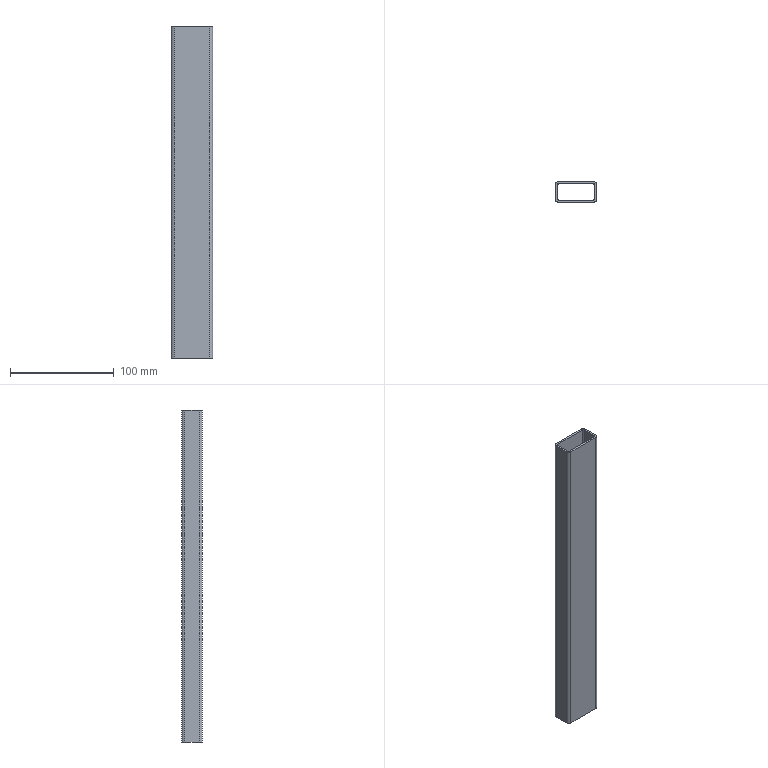Part | SolidWorks | features BaseBody 1 | 1 solid | 18 faces | box 40 x 20 x 320 mm | volume 69482 mm3 | plane 10 | cylinder 8 | commonest cylinder face diameters 2 x4 6 x4
STEP:
#1=CARTESIAN_POINT('',(18.,-7.,-160.));
#2=VERTEX_POINT('',#1);
#3=CARTESIAN_POINT('',(18.,7.,-160.));
#4=VERTEX_POINT('',#3);
#5=CARTESIAN_POINT('',(18.,7.,-160.));
#6=DIRECTION('',(0.,1.,0.));
#7=VECTOR('',#6,1000.);
#8=LINE('',#5,#7);
#9=EDGE_CURVE('',#2,#4,#8,.T.);
#10=ORIENTED_EDGE('',*,*,#9,.F.);
#11=CARTESIAN_POINT('',(18.,-7.,160.));
#12=VERTEX_POINT('',#11);
#13=CARTESIAN_POINT('',(18.,-7.,160.));
#14=DIRECTION('',(0.,0.,-1.));
#15=VECTOR('',#14,1000.);
#16=LINE('',#13,#15);
#17=EDGE_CURVE('',#12,#2,#16,.T.);
#18=ORIENTED_EDGE('',*,*,#17,.F.);
#19=CARTESIAN_POINT('',(18.,7.,160.));
#20=VERTEX_POINT('',#19);
#21=CARTESIAN_POINT('',(18.,7.,160.));
#22=DIRECTION('',(0.,1.,0.));
#23=VECTOR('',#22,1000.);
#24=LINE('',#21,#23);
#25=EDGE_CURVE('',#12,#20,#24,.T.);
#26=ORIENTED_EDGE('',*,*,#25,.T.);
#27=CARTESIAN_POINT('',(18.,7.,160.));
#28=DIRECTION('',(0.,0.,-1.));
#29=VECTOR('',#28,1000.);
#30=LINE('',#27,#29);
#31=EDGE_CURVE('',#20,#4,#30,.T.);
#32=ORIENTED_EDGE('',*,*,#31,.T.);
#33=EDGE_LOOP('',(#10,#18,#26,#32));
#34=FACE_OUTER_BOUND('',#33,.T.);
#35=CARTESIAN_POINT('',(18.,7.,160.));
#36=DIRECTION('',(-1.,0.,0.));
#37=DIRECTION('',(0.,0.,1.));
#38=AXIS2_PLACEMENT_3D('',#35,#36,#37);
#39=PLANE('',#38);
#40=ADVANCED_FACE('',(#34),#39,.T.);
#41=CARTESIAN_POINT('',(17.,-8.,-160.));
#42=VERTEX_POINT('',#41);
#43=CARTESIAN_POINT('',(17.,-7.,-160.));
#44=DIRECTION('',(0.,0.,1.));
#45=DIRECTION('',(1.,0.,0.));
#46=AXIS2_PLACEMENT_3D('',#43,#44,#45);
#47=CIRCLE('',#46,1.);
#48=EDGE_CURVE('',#42,#2,#47,.T.);
#49=ORIENTED_EDGE('',*,*,#48,.F.);
#50=CARTESIAN_POINT('',(17.,-8.,160.));
#51=VERTEX_POINT('',#50);
#52=CARTESIAN_POINT('',(17.,-8.,160.));
#53=DIRECTION('',(0.,0.,-1.));
#54=VECTOR('',#53,1000.);
#55=LINE('',#52,#54);
#56=EDGE_CURVE('',#51,#42,#55,.T.);
#57=ORIENTED_EDGE('',*,*,#56,.F.);
#58=CARTESIAN_POINT('',(17.,-7.,160.));
#59=DIRECTION('',(0.,0.,1.));
#60=DIRECTION('',(1.,0.,0.));
#61=AXIS2_PLACEMENT_3D('',#58,#59,#60);
#62=CIRCLE('',#61,1.);
#63=EDGE_CURVE('',#51,#12,#62,.T.);
#64=ORIENTED_EDGE('',*,*,#63,.T.);
#65=ORIENTED_EDGE('',*,*,#17,.T.);
#66=EDGE_LOOP('',(#49,#57,#64,#65));
#67=FACE_OUTER_BOUND('',#66,.T.);
#68=CARTESIAN_POINT('',(17.,-7.,160.));
#69=DIRECTION('',(0.,0.,-1.));
#70=DIRECTION('',(-1.,0.,0.));
#71=AXIS2_PLACEMENT_3D('',#68,#69,#70);
#72=CYLINDRICAL_SURFACE('',#71,1.);
#73=ADVANCED_FACE('',(#67),#72,.F.);
#74=CARTESIAN_POINT('',(-17.,-8.,-160.));
#75=VERTEX_POINT('',#74);
#76=CARTESIAN_POINT('',(-17.,-8.,-160.));
#77=DIRECTION('',(1.,0.,0.));
#78=VECTOR('',#77,1000.);
#79=LINE('',#76,#78);
#80=EDGE_CURVE('',#75,#42,#79,.T.);
#81=ORIENTED_EDGE('',*,*,#80,.F.);
#82=CARTESIAN_POINT('',(-17.,-8.,160.));
#83=VERTEX_POINT('',#82);
#84=CARTESIAN_POINT('',(-17.,-8.,160.));
#85=DIRECTION('',(0.,0.,-1.));
#86=VECTOR('',#85,1000.);
#87=LINE('',#84,#86);
#88=EDGE_CURVE('',#83,#75,#87,.T.);
#89=ORIENTED_EDGE('',*,*,#88,.F.);
#90=CARTESIAN_POINT('',(-17.,-8.,160.));
#91=DIRECTION('',(1.,0.,0.));
#92=VECTOR('',#91,1000.);
#93=LINE('',#90,#92);
#94=EDGE_CURVE('',#83,#51,#93,.T.);
#95=ORIENTED_EDGE('',*,*,#94,.T.);
#96=ORIENTED_EDGE('',*,*,#56,.T.);
#97=EDGE_LOOP('',(#81,#89,#95,#96));
#98=FACE_OUTER_BOUND('',#97,.T.);
#99=CARTESIAN_POINT('',(-17.,-8.,160.));
#100=DIRECTION('',(0.,1.,0.));
#101=DIRECTION('',(1.,0.,0.));
#102=AXIS2_PLACEMENT_3D('',#99,#100,#101);
#103=PLANE('',#102);
#104=ADVANCED_FACE('',(#98),#103,.T.);
#105=CARTESIAN_POINT('',(-18.,-7.,-160.));
#106=VERTEX_POINT('',#105);
#107=CARTESIAN_POINT('',(-17.,-7.,-160.));
#108=DIRECTION('',(0.,0.,1.));
#109=DIRECTION('',(1.,0.,0.));
#110=AXIS2_PLACEMENT_3D('',#107,#108,#109);
#111=CIRCLE('',#110,1.);
#112=EDGE_CURVE('',#106,#75,#111,.T.);
#113=ORIENTED_EDGE('',*,*,#112,.F.);
#114=CARTESIAN_POINT('',(-18.,-7.,160.));
#115=VERTEX_POINT('',#114);
#116=CARTESIAN_POINT('',(-18.,-7.,160.));
#117=DIRECTION('',(0.,0.,-1.));
#118=VECTOR('',#117,1000.);
#119=LINE('',#116,#118);
#120=EDGE_CURVE('',#115,#106,#119,.T.);
#121=ORIENTED_EDGE('',*,*,#120,.F.);
#122=CARTESIAN_POINT('',(-17.,-7.,160.));
#123=DIRECTION('',(0.,0.,1.));
#124=DIRECTION('',(1.,0.,0.));
#125=AXIS2_PLACEMENT_3D('',#122,#123,#124);
#126=CIRCLE('',#125,1.);
#127=EDGE_CURVE('',#115,#83,#126,.T.);
#128=ORIENTED_EDGE('',*,*,#127,.T.);
#129=ORIENTED_EDGE('',*,*,#88,.T.);
#130=EDGE_LOOP('',(#113,#121,#128,#129));
#131=FACE_OUTER_BOUND('',#130,.T.);
#132=CARTESIAN_POINT('',(-17.,-7.,160.));
#133=DIRECTION('',(0.,0.,-1.));
#134=DIRECTION('',(-1.,0.,0.));
#135=AXIS2_PLACEMENT_3D('',#132,#133,#134);
#136=CYLINDRICAL_SURFACE('',#135,1.);
#137=ADVANCED_FACE('',(#131),#136,.F.);
#138=CARTESIAN_POINT('',(-18.,7.,-160.));
#139=VERTEX_POINT('',#138);
#140=CARTESIAN_POINT('',(-18.,7.,-160.));
#141=DIRECTION('',(0.,-1.,0.));
#142=VECTOR('',#141,1000.);
#143=LINE('',#140,#142);
#144=EDGE_CURVE('',#139,#106,#143,.T.);
#145=ORIENTED_EDGE('',*,*,#144,.F.);
#146=CARTESIAN_POINT('',(-18.,7.,160.));
#147=VERTEX_POINT('',#146);
#148=CARTESIAN_POINT('',(-18.,7.,160.));
#149=DIRECTION('',(0.,0.,-1.));
#150=VECTOR('',#149,1000.);
#151=LINE('',#148,#150);
#152=EDGE_CURVE('',#147,#139,#151,.T.);
#153=ORIENTED_EDGE('',*,*,#152,.F.);
#154=CARTESIAN_POINT('',(-18.,7.,160.));
#155=DIRECTION('',(0.,-1.,0.));
#156=VECTOR('',#155,1000.);
#157=LINE('',#154,#156);
#158=EDGE_CURVE('',#147,#115,#157,.T.);
#159=ORIENTED_EDGE('',*,*,#158,.T.);
#160=ORIENTED_EDGE('',*,*,#120,.T.);
#161=EDGE_LOOP('',(#145,#153,#159,#160));
#162=FACE_OUTER_BOUND('',#161,.T.);
#163=CARTESIAN_POINT('',(-18.,7.,160.));
#164=DIRECTION('',(1.,0.,0.));
#165=DIRECTION('',(0.,-1.,0.));
#166=AXIS2_PLACEMENT_3D('',#163,#164,#165);
#167=PLANE('',#166);
#168=ADVANCED_FACE('',(#162),#167,.T.);
#169=CARTESIAN_POINT('',(-17.,8.,-160.));
#170=VERTEX_POINT('',#169);
#171=CARTESIAN_POINT('',(-17.,7.,-160.));
#172=DIRECTION('',(0.,0.,1.));
#173=DIRECTION('',(1.,0.,0.));
#174=AXIS2_PLACEMENT_3D('',#171,#172,#173);
#175=CIRCLE('',#174,1.);
#176=EDGE_CURVE('',#170,#139,#175,.T.);
#177=ORIENTED_EDGE('',*,*,#176,.F.);
#178=CARTESIAN_POINT('',(-17.,8.,160.));
#179=VERTEX_POINT('',#178);
#180=CARTESIAN_POINT('',(-17.,8.,160.));
#181=DIRECTION('',(0.,0.,-1.));
#182=VECTOR('',#181,1000.);
#183=LINE('',#180,#182);
#184=EDGE_CURVE('',#179,#170,#183,.T.);
#185=ORIENTED_EDGE('',*,*,#184,.F.);
#186=CARTESIAN_POINT('',(-17.,7.,160.));
#187=DIRECTION('',(0.,0.,1.));
#188=DIRECTION('',(1.,0.,0.));
#189=AXIS2_PLACEMENT_3D('',#186,#187,#188);
#190=CIRCLE('',#189,1.);
#191=EDGE_CURVE('',#179,#147,#190,.T.);
#192=ORIENTED_EDGE('',*,*,#191,.T.);
#193=ORIENTED_EDGE('',*,*,#152,.T.);
#194=EDGE_LOOP('',(#177,#185,#192,#193));
#195=FACE_OUTER_BOUND('',#194,.T.);
#196=CARTESIAN_POINT('',(-17.,7.,160.));
#197=DIRECTION('',(0.,0.,-1.));
#198=DIRECTION('',(-1.,0.,0.));
#199=AXIS2_PLACEMENT_3D('',#196,#197,#198);
#200=CYLINDRICAL_SURFACE('',#199,1.);
#201=ADVANCED_FACE('',(#195),#200,.F.);
#202=CARTESIAN_POINT('',(17.,8.,-160.));
#203=VERTEX_POINT('',#202);
#204=CARTESIAN_POINT('',(-17.,8.,-160.));
#205=DIRECTION('',(-1.,0.,0.));
#206=VECTOR('',#205,1000.);
#207=LINE('',#204,#206);
#208=EDGE_CURVE('',#203,#170,#207,.T.);
#209=ORIENTED_EDGE('',*,*,#208,.F.);
#210=CARTESIAN_POINT('',(17.,8.,160.));
#211=VERTEX_POINT('',#210);
#212=CARTESIAN_POINT('',(17.,8.,160.));
#213=DIRECTION('',(0.,0.,-1.));
#214=VECTOR('',#213,1000.);
#215=LINE('',#212,#214);
#216=EDGE_CURVE('',#211,#203,#215,.T.);
#217=ORIENTED_EDGE('',*,*,#216,.F.);
#218=CARTESIAN_POINT('',(-17.,8.,160.));
#219=DIRECTION('',(-1.,0.,0.));
#220=VECTOR('',#219,1000.);
#221=LINE('',#218,#220);
#222=EDGE_CURVE('',#211,#179,#221,.T.);
#223=ORIENTED_EDGE('',*,*,#222,.T.);
#224=ORIENTED_EDGE('',*,*,#184,.T.);
#225=EDGE_LOOP('',(#209,#217,#223,#224));
#226=FACE_OUTER_BOUND('',#225,.T.);
#227=CARTESIAN_POINT('',(-17.,8.,160.));
#228=DIRECTION('',(0.,-1.,0.));
#229=DIRECTION('',(0.,0.,-1.));
#230=AXIS2_PLACEMENT_3D('',#227,#228,#229);
#231=PLANE('',#230);
#232=ADVANCED_FACE('',(#226),#231,.T.);
#233=CARTESIAN_POINT('',(17.,7.,-160.));
#234=DIRECTION('',(0.,0.,1.));
#235=DIRECTION('',(-1.,0.,0.));
#236=AXIS2_PLACEMENT_3D('',#233,#234,#235);
#237=CIRCLE('',#236,1.);
#238=EDGE_CURVE('',#4,#203,#237,.T.);
#239=ORIENTED_EDGE('',*,*,#238,.F.);
#240=ORIENTED_EDGE('',*,*,#31,.F.);
#241=CARTESIAN_POINT('',(17.,7.,160.));
#242=DIRECTION('',(0.,0.,1.));
#243=DIRECTION('',(-1.,0.,0.));
#244=AXIS2_PLACEMENT_3D('',#241,#242,#243);
#245=CIRCLE('',#244,1.);
#246=EDGE_CURVE('',#20,#211,#245,.T.);
#247=ORIENTED_EDGE('',*,*,#246,.T.);
#248=ORIENTED_EDGE('',*,*,#216,.T.);
#249=EDGE_LOOP('',(#239,#240,#247,#248));
#250=FACE_OUTER_BOUND('',#249,.T.);
#251=CARTESIAN_POINT('',(17.,7.,160.));
#252=DIRECTION('',(0.,0.,-1.));
#253=DIRECTION('',(-1.,0.,0.));
#254=AXIS2_PLACEMENT_3D('',#251,#252,#253);
#255=CYLINDRICAL_SURFACE('',#254,1.);
#256=ADVANCED_FACE('',(#250),#255,.F.);
#257=CARTESIAN_POINT('',(-17.,-10.,-160.));
#258=VERTEX_POINT('',#257);
#259=CARTESIAN_POINT('',(17.,-10.,-160.));
#260=VERTEX_POINT('',#259);
#261=CARTESIAN_POINT('',(-17.,-10.,-160.));
#262=DIRECTION('',(1.,0.,0.));
#263=VECTOR('',#262,1000.);
#264=LINE('',#261,#263);
#265=EDGE_CURVE('',#258,#260,#264,.T.);
#266=ORIENTED_EDGE('',*,*,#265,.T.);
#267=CARTESIAN_POINT('',(17.,-10.,160.));
#268=VERTEX_POINT('',#267);
#269=CARTESIAN_POINT('',(17.,-10.,160.));
#270=DIRECTION('',(0.,0.,-1.));
#271=VECTOR('',#270,1000.);
#272=LINE('',#269,#271);
#273=EDGE_CURVE('',#268,#260,#272,.T.);
#274=ORIENTED_EDGE('',*,*,#273,.F.);
#275=CARTESIAN_POINT('',(-17.,-10.,160.));
#276=VERTEX_POINT('',#275);
#277=CARTESIAN_POINT('',(-17.,-10.,160.));
#278=DIRECTION('',(1.,0.,0.));
#279=VECTOR('',#278,1000.);
#280=LINE('',#277,#279);
#281=EDGE_CURVE('',#276,#268,#280,.T.);
#282=ORIENTED_EDGE('',*,*,#281,.F.);
#283=CARTESIAN_POINT('',(-17.,-10.,160.));
#284=DIRECTION('',(0.,0.,-1.));
#285=VECTOR('',#284,1000.);
#286=LINE('',#283,#285);
#287=EDGE_CURVE('',#276,#258,#286,.T.);
#288=ORIENTED_EDGE('',*,*,#287,.T.);
#289=EDGE_LOOP('',(#266,#274,#282,#288));
#290=FACE_OUTER_BOUND('',#289,.T.);
#291=CARTESIAN_POINT('',(-17.,-10.,160.));
#292=DIRECTION('',(0.,1.,0.));
#293=DIRECTION('',(1.,0.,0.));
#294=AXIS2_PLACEMENT_3D('',#291,#292,#293);
#295=PLANE('',#294);
#296=ADVANCED_FACE('',(#290),#295,.F.);
#297=CARTESIAN_POINT('',(-20.,-7.,-160.));
#298=VERTEX_POINT('',#297);
#299=CARTESIAN_POINT('',(-17.,-7.,-160.));
#300=DIRECTION('',(0.,0.,1.));
#301=DIRECTION('',(1.,0.,0.));
#302=AXIS2_PLACEMENT_3D('',#299,#300,#301);
#303=CIRCLE('',#302,3.);
#304=EDGE_CURVE('',#298,#258,#303,.T.);
#305=ORIENTED_EDGE('',*,*,#304,.T.);
#306=ORIENTED_EDGE('',*,*,#287,.F.);
#307=CARTESIAN_POINT('',(-20.,-7.,160.));
#308=VERTEX_POINT('',#307);
#309=CARTESIAN_POINT('',(-17.,-7.,160.));
#310=DIRECTION('',(0.,0.,1.));
#311=DIRECTION('',(1.,0.,0.));
#312=AXIS2_PLACEMENT_3D('',#309,#310,#311);
#313=CIRCLE('',#312,3.);
#314=EDGE_CURVE('',#308,#276,#313,.T.);
#315=ORIENTED_EDGE('',*,*,#314,.F.);
#316=CARTESIAN_POINT('',(-20.,-7.,160.));
#317=DIRECTION('',(0.,0.,-1.));
#318=VECTOR('',#317,1000.);
#319=LINE('',#316,#318);
#320=EDGE_CURVE('',#308,#298,#319,.T.);
#321=ORIENTED_EDGE('',*,*,#320,.T.);
#322=EDGE_LOOP('',(#305,#306,#315,#321));
#323=FACE_OUTER_BOUND('',#322,.T.);
#324=CARTESIAN_POINT('',(-17.,-7.,160.));
#325=DIRECTION('',(0.,0.,-1.));
#326=DIRECTION('',(-1.,0.,0.));
#327=AXIS2_PLACEMENT_3D('',#324,#325,#326);
#328=CYLINDRICAL_SURFACE('',#327,3.);
#329=ADVANCED_FACE('',(#323),#328,.T.);
#330=CARTESIAN_POINT('',(-20.,7.,-160.));
#331=VERTEX_POINT('',#330);
#332=CARTESIAN_POINT('',(-20.,7.,-160.));
#333=DIRECTION('',(0.,-1.,0.));
#334=VECTOR('',#333,1000.);
#335=LINE('',#332,#334);
#336=EDGE_CURVE('',#331,#298,#335,.T.);
#337=ORIENTED_EDGE('',*,*,#336,.T.);
#338=ORIENTED_EDGE('',*,*,#320,.F.);
#339=CARTESIAN_POINT('',(-20.,7.,160.));
#340=VERTEX_POINT('',#339);
#341=CARTESIAN_POINT('',(-20.,7.,160.));
#342=DIRECTION('',(0.,-1.,0.));
#343=VECTOR('',#342,1000.);
#344=LINE('',#341,#343);
#345=EDGE_CURVE('',#340,#308,#344,.T.);
#346=ORIENTED_EDGE('',*,*,#345,.F.);
#347=CARTESIAN_POINT('',(-20.,7.,160.));
#348=DIRECTION('',(0.,0.,-1.));
#349=VECTOR('',#348,1000.);
#350=LINE('',#347,#349);
#351=EDGE_CURVE('',#340,#331,#350,.T.);
#352=ORIENTED_EDGE('',*,*,#351,.T.);
#353=EDGE_LOOP('',(#337,#338,#346,#352));
#354=FACE_OUTER_BOUND('',#353,.T.);
#355=CARTESIAN_POINT('',(-20.,7.,160.));
#356=DIRECTION('',(1.,0.,0.));
#357=DIRECTION('',(0.,1.,0.));
#358=AXIS2_PLACEMENT_3D('',#355,#356,#357);
#359=PLANE('',#358);
#360=ADVANCED_FACE('',(#354),#359,.F.);
#361=CARTESIAN_POINT('',(-17.,10.,-160.));
#362=VERTEX_POINT('',#361);
#363=CARTESIAN_POINT('',(-17.,7.,-160.));
#364=DIRECTION('',(0.,0.,1.));
#365=DIRECTION('',(1.,0.,0.));
#366=AXIS2_PLACEMENT_3D('',#363,#364,#365);
#367=CIRCLE('',#366,3.);
#368=EDGE_CURVE('',#362,#331,#367,.T.);
#369=ORIENTED_EDGE('',*,*,#368,.T.);
#370=ORIENTED_EDGE('',*,*,#351,.F.);
#371=CARTESIAN_POINT('',(-17.,10.,160.));
#372=VERTEX_POINT('',#371);
#373=CARTESIAN_POINT('',(-17.,7.,160.));
#374=DIRECTION('',(0.,0.,1.));
#375=DIRECTION('',(1.,0.,0.));
#376=AXIS2_PLACEMENT_3D('',#373,#374,#375);
#377=CIRCLE('',#376,3.);
#378=EDGE_CURVE('',#372,#340,#377,.T.);
#379=ORIENTED_EDGE('',*,*,#378,.F.);
#380=CARTESIAN_POINT('',(-17.,10.,160.));
#381=DIRECTION('',(0.,0.,-1.));
#382=VECTOR('',#381,1000.);
#383=LINE('',#380,#382);
#384=EDGE_CURVE('',#372,#362,#383,.T.);
#385=ORIENTED_EDGE('',*,*,#384,.T.);
#386=EDGE_LOOP('',(#369,#370,#379,#385));
#387=FACE_OUTER_BOUND('',#386,.T.);
#388=CARTESIAN_POINT('',(-17.,7.,160.));
#389=DIRECTION('',(0.,0.,-1.));
#390=DIRECTION('',(-1.,0.,0.));
#391=AXIS2_PLACEMENT_3D('',#388,#389,#390);
#392=CYLINDRICAL_SURFACE('',#391,3.);
#393=ADVANCED_FACE('',(#387),#392,.T.);
#394=CARTESIAN_POINT('',(17.,10.,-160.));
#395=VERTEX_POINT('',#394);
#396=CARTESIAN_POINT('',(-17.,10.,-160.));
#397=DIRECTION('',(-1.,0.,0.));
#398=VECTOR('',#397,1000.);
#399=LINE('',#396,#398);
#400=EDGE_CURVE('',#395,#362,#399,.T.);
#401=ORIENTED_EDGE('',*,*,#400,.T.);
#402=ORIENTED_EDGE('',*,*,#384,.F.);
#403=CARTESIAN_POINT('',(17.,10.,160.));
#404=VERTEX_POINT('',#403);
#405=CARTESIAN_POINT('',(-17.,10.,160.));
#406=DIRECTION('',(-1.,0.,0.));
#407=VECTOR('',#406,1000.);
#408=LINE('',#405,#407);
#409=EDGE_CURVE('',#404,#372,#408,.T.);
#410=ORIENTED_EDGE('',*,*,#409,.F.);
#411=CARTESIAN_POINT('',(17.,10.,160.));
#412=DIRECTION('',(0.,0.,-1.));
#413=VECTOR('',#412,1000.);
#414=LINE('',#411,#413);
#415=EDGE_CURVE('',#404,#395,#414,.T.);
#416=ORIENTED_EDGE('',*,*,#415,.T.);
#417=EDGE_LOOP('',(#401,#402,#410,#416));
#418=FACE_OUTER_BOUND('',#417,.T.);
#419=CARTESIAN_POINT('',(-17.,10.,160.));
#420=DIRECTION('',(0.,-1.,0.));
#421=DIRECTION('',(0.,0.,-1.));
#422=AXIS2_PLACEMENT_3D('',#419,#420,#421);
#423=PLANE('',#422);
#424=ADVANCED_FACE('',(#418),#423,.F.);
#425=CARTESIAN_POINT('',(20.,7.,-160.));
#426=VERTEX_POINT('',#425);
#427=CARTESIAN_POINT('',(17.,7.,-160.));
#428=DIRECTION('',(0.,0.,1.));
#429=DIRECTION('',(-1.,0.,0.));
#430=AXIS2_PLACEMENT_3D('',#427,#428,#429);
#431=CIRCLE('',#430,3.);
#432=EDGE_CURVE('',#426,#395,#431,.T.);
#433=ORIENTED_EDGE('',*,*,#432,.T.);
#434=ORIENTED_EDGE('',*,*,#415,.F.);
#435=CARTESIAN_POINT('',(20.,7.,160.));
#436=VERTEX_POINT('',#435);
#437=CARTESIAN_POINT('',(17.,7.,160.));
#438=DIRECTION('',(0.,0.,1.));
#439=DIRECTION('',(-1.,0.,0.));
#440=AXIS2_PLACEMENT_3D('',#437,#438,#439);
#441=CIRCLE('',#440,3.);
#442=EDGE_CURVE('',#436,#404,#441,.T.);
#443=ORIENTED_EDGE('',*,*,#442,.F.);
#444=CARTESIAN_POINT('',(20.,7.,160.));
#445=DIRECTION('',(0.,0.,-1.));
#446=VECTOR('',#445,1000.);
#447=LINE('',#444,#446);
#448=EDGE_CURVE('',#436,#426,#447,.T.);
#449=ORIENTED_EDGE('',*,*,#448,.T.);
#450=EDGE_LOOP('',(#433,#434,#443,#449));
#451=FACE_OUTER_BOUND('',#450,.T.);
#452=CARTESIAN_POINT('',(17.,7.,160.));
#453=DIRECTION('',(0.,0.,-1.));
#454=DIRECTION('',(-1.,0.,0.));
#455=AXIS2_PLACEMENT_3D('',#452,#453,#454);
#456=CYLINDRICAL_SURFACE('',#455,3.);
#457=ADVANCED_FACE('',(#451),#456,.T.);
#458=CARTESIAN_POINT('',(20.,-7.,-160.));
#459=VERTEX_POINT('',#458);
#460=CARTESIAN_POINT('',(20.,7.,-160.));
#461=DIRECTION('',(0.,1.,0.));
#462=VECTOR('',#461,1000.);
#463=LINE('',#460,#462);
#464=EDGE_CURVE('',#459,#426,#463,.T.);
#465=ORIENTED_EDGE('',*,*,#464,.T.);
#466=ORIENTED_EDGE('',*,*,#448,.F.);
#467=CARTESIAN_POINT('',(20.,-7.,160.));
#468=VERTEX_POINT('',#467);
#469=CARTESIAN_POINT('',(20.,7.,160.));
#470=DIRECTION('',(0.,1.,0.));
#471=VECTOR('',#470,1000.);
#472=LINE('',#469,#471);
#473=EDGE_CURVE('',#468,#436,#472,.T.);
#474=ORIENTED_EDGE('',*,*,#473,.F.);
#475=CARTESIAN_POINT('',(20.,-7.,160.));
#476=DIRECTION('',(0.,0.,-1.));
#477=VECTOR('',#476,1000.);
#478=LINE('',#475,#477);
#479=EDGE_CURVE('',#468,#459,#478,.T.);
#480=ORIENTED_EDGE('',*,*,#479,.T.);
#481=EDGE_LOOP('',(#465,#466,#474,#480));
#482=FACE_OUTER_BOUND('',#481,.T.);
#483=CARTESIAN_POINT('',(20.,7.,160.));
#484=DIRECTION('',(-1.,0.,0.));
#485=DIRECTION('',(0.,0.,1.));
#486=AXIS2_PLACEMENT_3D('',#483,#484,#485);
#487=PLANE('',#486);
#488=ADVANCED_FACE('',(#482),#487,.F.);
#489=CARTESIAN_POINT('',(17.,-7.,-160.));
#490=DIRECTION('',(0.,0.,1.));
#491=DIRECTION('',(1.,0.,0.));
#492=AXIS2_PLACEMENT_3D('',#489,#490,#491);
#493=CIRCLE('',#492,3.);
#494=EDGE_CURVE('',#260,#459,#493,.T.);
#495=ORIENTED_EDGE('',*,*,#494,.T.);
#496=ORIENTED_EDGE('',*,*,#479,.F.);
#497=CARTESIAN_POINT('',(17.,-7.,160.));
#498=DIRECTION('',(0.,0.,1.));
#499=DIRECTION('',(1.,0.,0.));
#500=AXIS2_PLACEMENT_3D('',#497,#498,#499);
#501=CIRCLE('',#500,3.);
#502=EDGE_CURVE('',#268,#468,#501,.T.);
#503=ORIENTED_EDGE('',*,*,#502,.F.);
#504=ORIENTED_EDGE('',*,*,#273,.T.);
#505=EDGE_LOOP('',(#495,#496,#503,#504));
#506=FACE_OUTER_BOUND('',#505,.T.);
#507=CARTESIAN_POINT('',(17.,-7.,160.));
#508=DIRECTION('',(0.,0.,-1.));
#509=DIRECTION('',(-1.,0.,0.));
#510=AXIS2_PLACEMENT_3D('',#507,#508,#509);
#511=CYLINDRICAL_SURFACE('',#510,3.);
#512=ADVANCED_FACE('',(#506),#511,.T.);
#513=ORIENTED_EDGE('',*,*,#238,.T.);
#514=ORIENTED_EDGE('',*,*,#208,.T.);
#515=ORIENTED_EDGE('',*,*,#176,.T.);
#516=ORIENTED_EDGE('',*,*,#144,.T.);
#517=ORIENTED_EDGE('',*,*,#112,.T.);
#518=ORIENTED_EDGE('',*,*,#80,.T.);
#519=ORIENTED_EDGE('',*,*,#48,.T.);
#520=ORIENTED_EDGE('',*,*,#9,.T.);
#521=EDGE_LOOP('',(#513,#514,#515,#516,#517,#518,#519,#520));
#522=FACE_BOUND('',#521,.T.);
#523=ORIENTED_EDGE('',*,*,#494,.F.);
#524=ORIENTED_EDGE('',*,*,#265,.F.);
#525=ORIENTED_EDGE('',*,*,#304,.F.);
#526=ORIENTED_EDGE('',*,*,#336,.F.);
#527=ORIENTED_EDGE('',*,*,#368,.F.);
#528=ORIENTED_EDGE('',*,*,#400,.F.);
#529=ORIENTED_EDGE('',*,*,#432,.F.);
#530=ORIENTED_EDGE('',*,*,#464,.F.);
#531=EDGE_LOOP('',(#523,#524,#525,#526,#527,#528,#529,#530));
#532=FACE_OUTER_BOUND('',#531,.T.);
#533=CARTESIAN_POINT('',(17.,-7.,-160.));
#534=DIRECTION('',(0.,0.,1.));
#535=DIRECTION('',(1.,0.,0.));
#536=AXIS2_PLACEMENT_3D('',#533,#534,#535);
#537=PLANE('',#536);
#538=ADVANCED_FACE('',(#522,#532),#537,.F.);
#539=ORIENTED_EDGE('',*,*,#222,.F.);
#540=ORIENTED_EDGE('',*,*,#246,.F.);
#541=ORIENTED_EDGE('',*,*,#25,.F.);
#542=ORIENTED_EDGE('',*,*,#63,.F.);
#543=ORIENTED_EDGE('',*,*,#94,.F.);
#544=ORIENTED_EDGE('',*,*,#127,.F.);
#545=ORIENTED_EDGE('',*,*,#158,.F.);
#546=ORIENTED_EDGE('',*,*,#191,.F.);
#547=EDGE_LOOP('',(#539,#540,#541,#542,#543,#544,#545,#546));
#548=FACE_BOUND('',#547,.T.);
#549=ORIENTED_EDGE('',*,*,#502,.T.);
#550=ORIENTED_EDGE('',*,*,#473,.T.);
#551=ORIENTED_EDGE('',*,*,#442,.T.);
#552=ORIENTED_EDGE('',*,*,#409,.T.);
#553=ORIENTED_EDGE('',*,*,#378,.T.);
#554=ORIENTED_EDGE('',*,*,#345,.T.);
#555=ORIENTED_EDGE('',*,*,#314,.T.);
#556=ORIENTED_EDGE('',*,*,#281,.T.);
#557=EDGE_LOOP('',(#549,#550,#551,#552,#553,#554,#555,#556));
#558=FACE_OUTER_BOUND('',#557,.T.);
#559=CARTESIAN_POINT('',(17.,-7.,160.));
#560=DIRECTION('',(0.,0.,1.));
#561=DIRECTION('',(1.,0.,0.));
#562=AXIS2_PLACEMENT_3D('',#559,#560,#561);
#563=PLANE('',#562);
#564=ADVANCED_FACE('',(#548,#558),#563,.T.);
#565=CLOSED_SHELL('',(#40,#73,#104,#137,#168,#201,#232,#256,#296,#329,#360,#393,#424,#457,#488,#512,#538,#564));
#566=MANIFOLD_SOLID_BREP('',#565);
#567=CARTESIAN_POINT('',(0.,0.,0.));
#568=DIRECTION('',(0.,0.,1.));
#569=DIRECTION('',(1.,0.,0.));
#570=AXIS2_PLACEMENT_3D('',#567,#568,#569);
#571=(LENGTH_UNIT()NAMED_UNIT(*)SI_UNIT(.MILLI.,.METRE.));
#572=UNCERTAINTY_MEASURE_WITH_UNIT(LENGTH_MEASURE(0.00001),#571,'','');
#573=(NAMED_UNIT(*)PLANE_ANGLE_UNIT()SI_UNIT($,.RADIAN.));
#574=(NAMED_UNIT(*)SI_UNIT($,.STERADIAN.)SOLID_ANGLE_UNIT());
#575=(GEOMETRIC_REPRESENTATION_CONTEXT(3)GLOBAL_UNCERTAINTY_ASSIGNED_CONTEXT((#572))GLOBAL_UNIT_ASSIGNED_CONTEXT((#571,#573,#574))REPRESENTATION_CONTEXT('',''));
#576=ADVANCED_BREP_SHAPE_REPRESENTATION('',(#566,#570),#575);